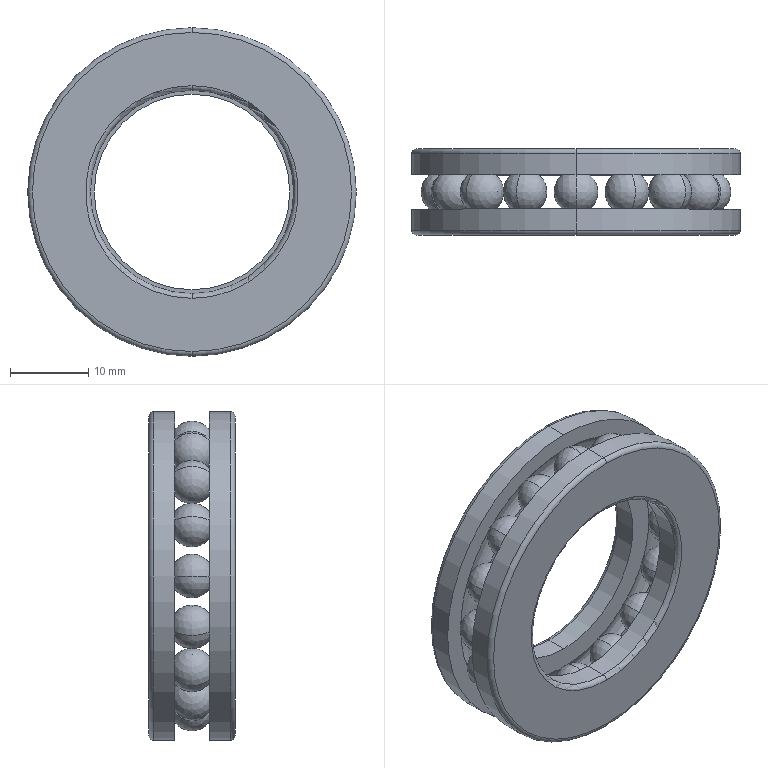Part | SolidWorks | features Revolution 3, CirPattern 1, Fillet 1 | 1 solid | 86 faces | box 42 x 11 x 42 mm | volume 6942 mm3 | torus 40 | sphere 32 | cylinder 8 | plane 6 | commonest cylinder face diameters 42 x4 25 x2 26 x2